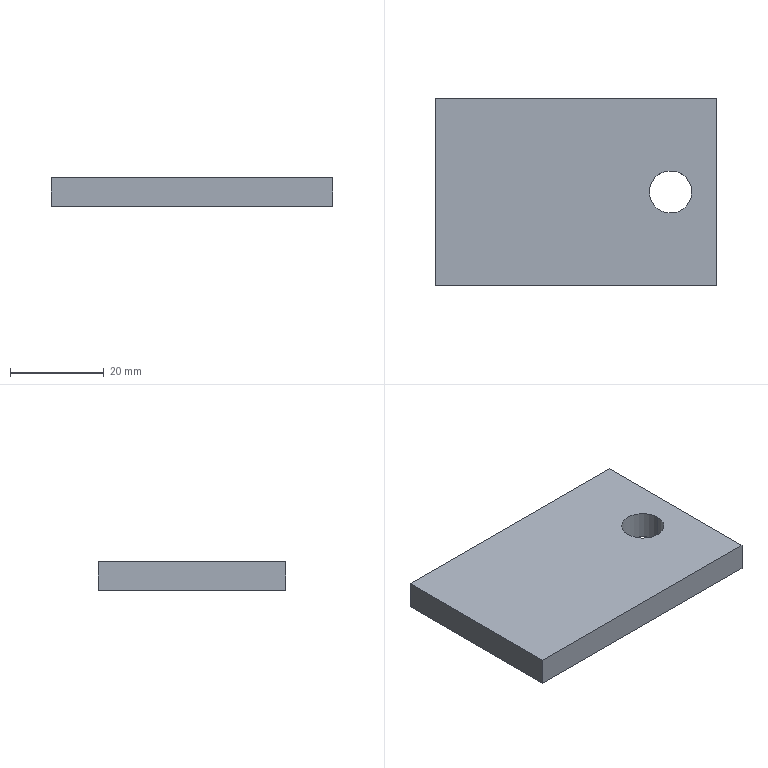Part | SolidWorks | features Extrusion 1, ICE 1 | 1 solid | 8 faces | box 60 x 40 x 6 mm | volume 14018 mm3 | plane 6 | cylinder 2 | commonest cylinder face diameters 9 x2
STEP:
#1=CARTESIAN_POINT('',(15.635,0.,0.));
#2=VERTEX_POINT('',#1);
#3=CARTESIAN_POINT('',(24.635,0.,0.));
#4=VERTEX_POINT('',#3);
#5=CARTESIAN_POINT('',(20.135,0.,0.));
#6=DIRECTION('',(0.,0.,1.));
#7=DIRECTION('',(1.,0.,0.));
#8=AXIS2_PLACEMENT_3D('',#5,#6,#7);
#9=CIRCLE('',#8,4.5);
#10=EDGE_CURVE('',#2,#4,#9,.T.);
#11=ORIENTED_EDGE('',*,*,#10,.F.);
#12=CARTESIAN_POINT('',(15.635,0.,6.));
#13=VERTEX_POINT('',#12);
#14=CARTESIAN_POINT('',(15.635,0.,0.));
#15=DIRECTION('',(0.,0.,1.));
#16=VECTOR('',#15,1000.);
#17=LINE('',#14,#16);
#18=EDGE_CURVE('',#2,#13,#17,.T.);
#19=ORIENTED_EDGE('',*,*,#18,.T.);
#20=CARTESIAN_POINT('',(24.635,0.,6.));
#21=VERTEX_POINT('',#20);
#22=CARTESIAN_POINT('',(20.135,0.,6.));
#23=DIRECTION('',(0.,0.,1.));
#24=DIRECTION('',(1.,0.,0.));
#25=AXIS2_PLACEMENT_3D('',#22,#23,#24);
#26=CIRCLE('',#25,4.5);
#27=EDGE_CURVE('',#13,#21,#26,.T.);
#28=ORIENTED_EDGE('',*,*,#27,.T.);
#29=CARTESIAN_POINT('',(24.635,0.,0.));
#30=DIRECTION('',(0.,0.,1.));
#31=VECTOR('',#30,1000.);
#32=LINE('',#29,#31);
#33=EDGE_CURVE('',#4,#21,#32,.T.);
#34=ORIENTED_EDGE('',*,*,#33,.F.);
#35=EDGE_LOOP('',(#11,#19,#28,#34));
#36=FACE_OUTER_BOUND('',#35,.T.);
#37=CARTESIAN_POINT('',(20.135,0.,0.));
#38=DIRECTION('',(0.,0.,1.));
#39=DIRECTION('',(1.,0.,0.));
#40=AXIS2_PLACEMENT_3D('',#37,#38,#39);
#41=CYLINDRICAL_SURFACE('',#40,4.5);
#42=ADVANCED_FACE('',(#36),#41,.F.);
#43=CARTESIAN_POINT('',(30.,-20.,0.));
#44=VERTEX_POINT('',#43);
#45=CARTESIAN_POINT('',(30.,20.,0.));
#46=VERTEX_POINT('',#45);
#47=CARTESIAN_POINT('',(30.,-20.,0.));
#48=DIRECTION('',(0.,1.,0.));
#49=VECTOR('',#48,1000.);
#50=LINE('',#47,#49);
#51=EDGE_CURVE('',#44,#46,#50,.T.);
#52=ORIENTED_EDGE('',*,*,#51,.T.);
#53=CARTESIAN_POINT('',(30.,20.,6.));
#54=VERTEX_POINT('',#53);
#55=CARTESIAN_POINT('',(30.,20.,6.));
#56=DIRECTION('',(0.,0.,-1.));
#57=VECTOR('',#56,1000.);
#58=LINE('',#55,#57);
#59=EDGE_CURVE('',#54,#46,#58,.T.);
#60=ORIENTED_EDGE('',*,*,#59,.F.);
#61=CARTESIAN_POINT('',(30.,-20.,6.));
#62=VERTEX_POINT('',#61);
#63=CARTESIAN_POINT('',(30.,-20.,6.));
#64=DIRECTION('',(0.,1.,0.));
#65=VECTOR('',#64,1000.);
#66=LINE('',#63,#65);
#67=EDGE_CURVE('',#62,#54,#66,.T.);
#68=ORIENTED_EDGE('',*,*,#67,.F.);
#69=CARTESIAN_POINT('',(30.,-20.,6.));
#70=DIRECTION('',(0.,0.,-1.));
#71=VECTOR('',#70,1000.);
#72=LINE('',#69,#71);
#73=EDGE_CURVE('',#62,#44,#72,.T.);
#74=ORIENTED_EDGE('',*,*,#73,.T.);
#75=EDGE_LOOP('',(#52,#60,#68,#74));
#76=FACE_OUTER_BOUND('',#75,.T.);
#77=CARTESIAN_POINT('',(30.,-20.,6.));
#78=DIRECTION('',(-1.,0.,0.));
#79=DIRECTION('',(0.,0.,1.));
#80=AXIS2_PLACEMENT_3D('',#77,#78,#79);
#81=PLANE('',#80);
#82=ADVANCED_FACE('',(#76),#81,.F.);
#83=CARTESIAN_POINT('',(-30.,20.,0.));
#84=VERTEX_POINT('',#83);
#85=CARTESIAN_POINT('',(-30.,20.,0.));
#86=DIRECTION('',(-1.,0.,0.));
#87=VECTOR('',#86,1000.);
#88=LINE('',#85,#87);
#89=EDGE_CURVE('',#46,#84,#88,.T.);
#90=ORIENTED_EDGE('',*,*,#89,.T.);
#91=CARTESIAN_POINT('',(-30.,20.,6.));
#92=VERTEX_POINT('',#91);
#93=CARTESIAN_POINT('',(-30.,20.,6.));
#94=DIRECTION('',(0.,0.,-1.));
#95=VECTOR('',#94,1000.);
#96=LINE('',#93,#95);
#97=EDGE_CURVE('',#92,#84,#96,.T.);
#98=ORIENTED_EDGE('',*,*,#97,.F.);
#99=CARTESIAN_POINT('',(-30.,20.,6.));
#100=DIRECTION('',(-1.,0.,0.));
#101=VECTOR('',#100,1000.);
#102=LINE('',#99,#101);
#103=EDGE_CURVE('',#54,#92,#102,.T.);
#104=ORIENTED_EDGE('',*,*,#103,.F.);
#105=ORIENTED_EDGE('',*,*,#59,.T.);
#106=EDGE_LOOP('',(#90,#98,#104,#105));
#107=FACE_OUTER_BOUND('',#106,.T.);
#108=CARTESIAN_POINT('',(-30.,20.,6.));
#109=DIRECTION('',(0.,-1.,0.));
#110=DIRECTION('',(0.,0.,-1.));
#111=AXIS2_PLACEMENT_3D('',#108,#109,#110);
#112=PLANE('',#111);
#113=ADVANCED_FACE('',(#107),#112,.F.);
#114=CARTESIAN_POINT('',(-30.,-20.,0.));
#115=VERTEX_POINT('',#114);
#116=CARTESIAN_POINT('',(-30.,-20.,0.));
#117=DIRECTION('',(0.,-1.,0.));
#118=VECTOR('',#117,1000.);
#119=LINE('',#116,#118);
#120=EDGE_CURVE('',#84,#115,#119,.T.);
#121=ORIENTED_EDGE('',*,*,#120,.T.);
#122=CARTESIAN_POINT('',(-30.,-20.,6.));
#123=VERTEX_POINT('',#122);
#124=CARTESIAN_POINT('',(-30.,-20.,6.));
#125=DIRECTION('',(0.,0.,-1.));
#126=VECTOR('',#125,1000.);
#127=LINE('',#124,#126);
#128=EDGE_CURVE('',#123,#115,#127,.T.);
#129=ORIENTED_EDGE('',*,*,#128,.F.);
#130=CARTESIAN_POINT('',(-30.,-20.,6.));
#131=DIRECTION('',(0.,-1.,0.));
#132=VECTOR('',#131,1000.);
#133=LINE('',#130,#132);
#134=EDGE_CURVE('',#92,#123,#133,.T.);
#135=ORIENTED_EDGE('',*,*,#134,.F.);
#136=ORIENTED_EDGE('',*,*,#97,.T.);
#137=EDGE_LOOP('',(#121,#129,#135,#136));
#138=FACE_OUTER_BOUND('',#137,.T.);
#139=CARTESIAN_POINT('',(-30.,-20.,6.));
#140=DIRECTION('',(1.,0.,0.));
#141=DIRECTION('',(0.,0.,-1.));
#142=AXIS2_PLACEMENT_3D('',#139,#140,#141);
#143=PLANE('',#142);
#144=ADVANCED_FACE('',(#138),#143,.F.);
#145=CARTESIAN_POINT('',(-30.,-20.,0.));
#146=DIRECTION('',(1.,0.,0.));
#147=VECTOR('',#146,1000.);
#148=LINE('',#145,#147);
#149=EDGE_CURVE('',#115,#44,#148,.T.);
#150=ORIENTED_EDGE('',*,*,#149,.T.);
#151=ORIENTED_EDGE('',*,*,#73,.F.);
#152=CARTESIAN_POINT('',(-30.,-20.,6.));
#153=DIRECTION('',(1.,0.,0.));
#154=VECTOR('',#153,1000.);
#155=LINE('',#152,#154);
#156=EDGE_CURVE('',#123,#62,#155,.T.);
#157=ORIENTED_EDGE('',*,*,#156,.F.);
#158=ORIENTED_EDGE('',*,*,#128,.T.);
#159=EDGE_LOOP('',(#150,#151,#157,#158));
#160=FACE_OUTER_BOUND('',#159,.T.);
#161=CARTESIAN_POINT('',(-30.,-20.,6.));
#162=DIRECTION('',(0.,1.,0.));
#163=DIRECTION('',(0.,0.,1.));
#164=AXIS2_PLACEMENT_3D('',#161,#162,#163);
#165=PLANE('',#164);
#166=ADVANCED_FACE('',(#160),#165,.F.);
#167=CARTESIAN_POINT('',(20.135,0.,6.));
#168=DIRECTION('',(0.,0.,1.));
#169=DIRECTION('',(1.,0.,0.));
#170=AXIS2_PLACEMENT_3D('',#167,#168,#169);
#171=CIRCLE('',#170,4.5);
#172=EDGE_CURVE('',#21,#13,#171,.T.);
#173=ORIENTED_EDGE('',*,*,#172,.F.);
#174=ORIENTED_EDGE('',*,*,#27,.F.);
#175=EDGE_LOOP('',(#173,#174));
#176=FACE_BOUND('',#175,.T.);
#177=ORIENTED_EDGE('',*,*,#67,.T.);
#178=ORIENTED_EDGE('',*,*,#103,.T.);
#179=ORIENTED_EDGE('',*,*,#134,.T.);
#180=ORIENTED_EDGE('',*,*,#156,.T.);
#181=EDGE_LOOP('',(#177,#178,#179,#180));
#182=FACE_OUTER_BOUND('',#181,.T.);
#183=CARTESIAN_POINT('',(0.,0.,6.));
#184=DIRECTION('',(0.,0.,-1.));
#185=DIRECTION('',(-1.,0.,0.));
#186=AXIS2_PLACEMENT_3D('',#183,#184,#185);
#187=PLANE('',#186);
#188=ADVANCED_FACE('',(#176,#182),#187,.F.);
#189=CARTESIAN_POINT('',(20.135,0.,0.));
#190=DIRECTION('',(0.,0.,1.));
#191=DIRECTION('',(1.,0.,0.));
#192=AXIS2_PLACEMENT_3D('',#189,#190,#191);
#193=CIRCLE('',#192,4.5);
#194=EDGE_CURVE('',#4,#2,#193,.T.);
#195=ORIENTED_EDGE('',*,*,#194,.T.);
#196=ORIENTED_EDGE('',*,*,#10,.T.);
#197=EDGE_LOOP('',(#195,#196));
#198=FACE_BOUND('',#197,.T.);
#199=ORIENTED_EDGE('',*,*,#51,.F.);
#200=ORIENTED_EDGE('',*,*,#149,.F.);
#201=ORIENTED_EDGE('',*,*,#120,.F.);
#202=ORIENTED_EDGE('',*,*,#89,.F.);
#203=EDGE_LOOP('',(#199,#200,#201,#202));
#204=FACE_OUTER_BOUND('',#203,.T.);
#205=CARTESIAN_POINT('',(0.,0.,0.));
#206=DIRECTION('',(0.,0.,-1.));
#207=DIRECTION('',(-1.,0.,0.));
#208=AXIS2_PLACEMENT_3D('',#205,#206,#207);
#209=PLANE('',#208);
#210=ADVANCED_FACE('',(#198,#204),#209,.T.);
#211=ORIENTED_EDGE('',*,*,#18,.F.);
#212=ORIENTED_EDGE('',*,*,#194,.F.);
#213=ORIENTED_EDGE('',*,*,#33,.T.);
#214=ORIENTED_EDGE('',*,*,#172,.T.);
#215=EDGE_LOOP('',(#211,#212,#213,#214));
#216=FACE_OUTER_BOUND('',#215,.T.);
#217=CARTESIAN_POINT('',(20.135,0.,0.));
#218=DIRECTION('',(0.,0.,1.));
#219=DIRECTION('',(1.,0.,0.));
#220=AXIS2_PLACEMENT_3D('',#217,#218,#219);
#221=CYLINDRICAL_SURFACE('',#220,4.5);
#222=ADVANCED_FACE('',(#216),#221,.F.);
#223=CLOSED_SHELL('',(#42,#82,#113,#144,#166,#188,#210,#222));
#224=MANIFOLD_SOLID_BREP('',#223);
#225=CARTESIAN_POINT('',(0.,0.,0.));
#226=DIRECTION('',(0.,0.,1.));
#227=DIRECTION('',(1.,0.,0.));
#228=AXIS2_PLACEMENT_3D('',#225,#226,#227);
#229=(LENGTH_UNIT()NAMED_UNIT(*)SI_UNIT(.MILLI.,.METRE.));
#230=UNCERTAINTY_MEASURE_WITH_UNIT(LENGTH_MEASURE(0.00001),#229,'','');
#231=(NAMED_UNIT(*)PLANE_ANGLE_UNIT()SI_UNIT($,.RADIAN.));
#232=(NAMED_UNIT(*)SI_UNIT($,.STERADIAN.)SOLID_ANGLE_UNIT());
#233=(GEOMETRIC_REPRESENTATION_CONTEXT(3)GLOBAL_UNCERTAINTY_ASSIGNED_CONTEXT((#230))GLOBAL_UNIT_ASSIGNED_CONTEXT((#229,#231,#232))REPRESENTATION_CONTEXT('',''));
#234=ADVANCED_BREP_SHAPE_REPRESENTATION('',(#224,#228),#233);